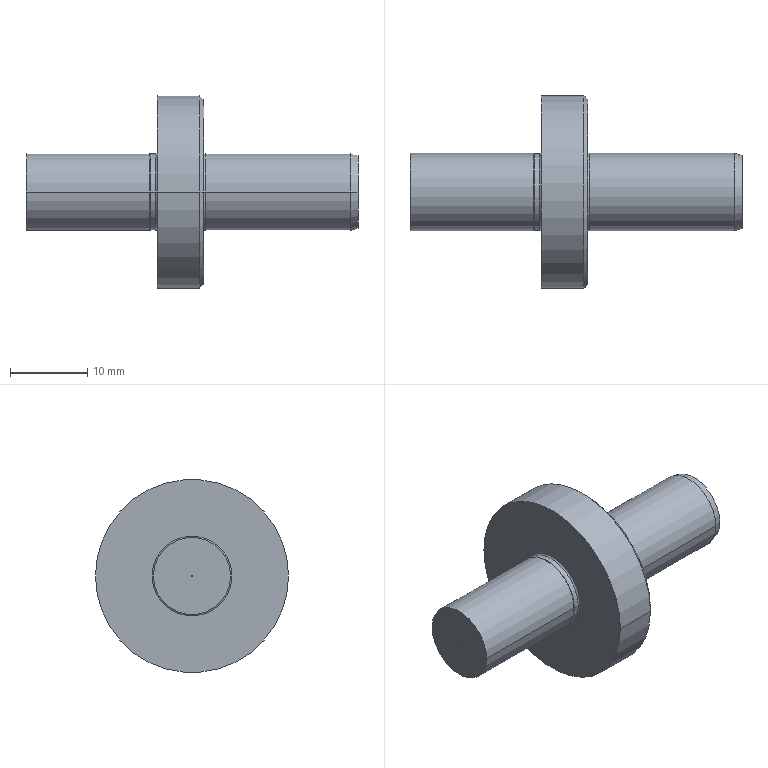Part | SolidWorks | features ICE 5, RevCut 5, Revolution 4, Fillet 2, Chamfer 1, DelFace 1, RefAxis 1 | 1 solid | 26 faces | box 43 x 25 x 25 mm | volume 5837 mm3 | cone 8 | cylinder 8 | torus 6 | plane 4 | commonest cylinder face diameters 10 x4 9.95 x2 25 x2
STEP:
#1=CARTESIAN_POINT('',(25.9,0.,0.));
#2=VERTEX_POINT('',#1);
#3=CARTESIAN_POINT('',(26.,0.,-0.1));
#4=VERTEX_POINT('',#3);
#5=CARTESIAN_POINT('',(26.,0.,-0.1));
#6=DIRECTION('',(0.7071,0.,-0.7071));
#7=VECTOR('',#6,1000.);
#8=LINE('',#5,#7);
#9=EDGE_CURVE('',#2,#4,#8,.T.);
#10=ORIENTED_EDGE('',*,*,#9,.F.);
#11=CARTESIAN_POINT('',(26.,0.,0.1));
#12=VERTEX_POINT('',#11);
#13=CARTESIAN_POINT('',(26.,0.,0.1));
#14=DIRECTION('',(0.7071,0.,0.7071));
#15=VECTOR('',#14,1000.);
#16=LINE('',#13,#15);
#17=EDGE_CURVE('',#2,#12,#16,.T.);
#18=ORIENTED_EDGE('',*,*,#17,.T.);
#19=CARTESIAN_POINT('',(26.,0.,0.));
#20=DIRECTION('',(-1.,0.,0.));
#21=DIRECTION('',(0.,0.,1.));
#22=AXIS2_PLACEMENT_3D('',#19,#20,#21);
#23=CIRCLE('',#22,0.1);
#24=EDGE_CURVE('',#4,#12,#23,.T.);
#25=ORIENTED_EDGE('',*,*,#24,.F.);
#26=EDGE_LOOP('',(#10,#18,#25));
#27=FACE_OUTER_BOUND('',#26,.T.);
#28=CARTESIAN_POINT('',(26.,0.,0.));
#29=DIRECTION('',(1.,0.,0.));
#30=DIRECTION('',(0.,0.,-1.));
#31=AXIS2_PLACEMENT_3D('',#28,#29,#30);
#32=CONICAL_SURFACE('',#31,0.1,0.7854);
#33=ADVANCED_FACE('',(#27),#32,.F.);
#34=CARTESIAN_POINT('',(26.,-4.732,0.));
#35=VERTEX_POINT('',#34);
#36=CARTESIAN_POINT('',(26.,4.732,0.));
#37=VERTEX_POINT('',#36);
#38=CARTESIAN_POINT('',(26.,0.,0.));
#39=DIRECTION('',(-1.,0.,0.));
#40=DIRECTION('',(0.,-1.,0.));
#41=AXIS2_PLACEMENT_3D('',#38,#39,#40);
#42=CIRCLE('',#41,4.732);
#43=EDGE_CURVE('',#35,#37,#42,.T.);
#44=ORIENTED_EDGE('',*,*,#43,.T.);
#45=CARTESIAN_POINT('',(25.,5.,0.));
#46=VERTEX_POINT('',#45);
#47=CARTESIAN_POINT('',(26.,4.732,0.));
#48=DIRECTION('',(-0.9659,0.2588,0.));
#49=VECTOR('',#48,1000.);
#50=LINE('',#47,#49);
#51=EDGE_CURVE('',#37,#46,#50,.T.);
#52=ORIENTED_EDGE('',*,*,#51,.T.);
#53=CARTESIAN_POINT('',(25.,-5.,0.));
#54=VERTEX_POINT('',#53);
#55=CARTESIAN_POINT('',(25.,0.,0.));
#56=DIRECTION('',(-1.,0.,0.));
#57=DIRECTION('',(0.,-1.,0.));
#58=AXIS2_PLACEMENT_3D('',#55,#56,#57);
#59=CIRCLE('',#58,5.);
#60=EDGE_CURVE('',#54,#46,#59,.T.);
#61=ORIENTED_EDGE('',*,*,#60,.F.);
#62=CARTESIAN_POINT('',(26.,-4.732,0.));
#63=DIRECTION('',(-0.9659,-0.2588,0.));
#64=VECTOR('',#63,1000.);
#65=LINE('',#62,#64);
#66=EDGE_CURVE('',#35,#54,#65,.T.);
#67=ORIENTED_EDGE('',*,*,#66,.F.);
#68=EDGE_LOOP('',(#44,#52,#61,#67));
#69=FACE_OUTER_BOUND('',#68,.T.);
#70=CARTESIAN_POINT('',(26.,0.,0.));
#71=DIRECTION('',(-1.,0.,0.));
#72=DIRECTION('',(0.,-1.,0.));
#73=AXIS2_PLACEMENT_3D('',#70,#71,#72);
#74=CONICAL_SURFACE('',#73,4.732,0.2618);
#75=ADVANCED_FACE('',(#69),#74,.T.);
#76=CARTESIAN_POINT('',(-1.,5.,0.));
#77=VERTEX_POINT('',#76);
#78=CARTESIAN_POINT('',(-1.,-5.,0.));
#79=VERTEX_POINT('',#78);
#80=CARTESIAN_POINT('',(-1.,0.,0.));
#81=DIRECTION('',(-1.,0.,0.));
#82=DIRECTION('',(0.,-1.,0.));
#83=AXIS2_PLACEMENT_3D('',#80,#81,#82);
#84=CIRCLE('',#83,5.);
#85=EDGE_CURVE('',#77,#79,#84,.T.);
#86=ORIENTED_EDGE('',*,*,#85,.F.);
#87=CARTESIAN_POINT('',(-0.9032,4.975,0.));
#88=VERTEX_POINT('',#87);
#89=CARTESIAN_POINT('',(-0.9032,5.175,0.));
#90=DIRECTION('',(0.,0.,1.));
#91=DIRECTION('',(0.,-1.,0.));
#92=AXIS2_PLACEMENT_3D('',#89,#90,#91);
#93=CIRCLE('',#92,0.2);
#94=EDGE_CURVE('',#77,#88,#93,.T.);
#95=ORIENTED_EDGE('',*,*,#94,.T.);
#96=CARTESIAN_POINT('',(-0.9032,-4.975,0.));
#97=VERTEX_POINT('',#96);
#98=CARTESIAN_POINT('',(-0.9032,0.,0.));
#99=DIRECTION('',(1.,0.,0.));
#100=DIRECTION('',(0.,-1.,0.));
#101=AXIS2_PLACEMENT_3D('',#98,#99,#100);
#102=CIRCLE('',#101,4.975);
#103=EDGE_CURVE('',#97,#88,#102,.T.);
#104=ORIENTED_EDGE('',*,*,#103,.F.);
#105=CARTESIAN_POINT('',(-0.9032,-5.175,0.));
#106=DIRECTION('',(0.,0.,-1.));
#107=DIRECTION('',(-1.,0.,0.));
#108=AXIS2_PLACEMENT_3D('',#105,#106,#107);
#109=CIRCLE('',#108,0.2);
#110=EDGE_CURVE('',#79,#97,#109,.T.);
#111=ORIENTED_EDGE('',*,*,#110,.F.);
#112=EDGE_LOOP('',(#86,#95,#104,#111));
#113=FACE_OUTER_BOUND('',#112,.T.);
#114=CARTESIAN_POINT('',(-0.9032,0.,0.));
#115=DIRECTION('',(-1.,0.,0.));
#116=DIRECTION('',(0.,-1.,0.));
#117=AXIS2_PLACEMENT_3D('',#114,#115,#116);
#118=TOROIDAL_SURFACE('',#117,5.175,0.2);
#119=ADVANCED_FACE('',(#113),#118,.F.);
#120=CARTESIAN_POINT('',(0.,-5.175,0.));
#121=VERTEX_POINT('',#120);
#122=CARTESIAN_POINT('',(0.,5.175,0.));
#123=VERTEX_POINT('',#122);
#124=CARTESIAN_POINT('',(0.,0.,0.));
#125=DIRECTION('',(1.,0.,0.));
#126=DIRECTION('',(0.,1.,0.));
#127=AXIS2_PLACEMENT_3D('',#124,#125,#126);
#128=CIRCLE('',#127,5.175);
#129=EDGE_CURVE('',#121,#123,#128,.T.);
#130=ORIENTED_EDGE('',*,*,#129,.F.);
#131=CARTESIAN_POINT('',(-0.2,-4.975,0.));
#132=VERTEX_POINT('',#131);
#133=CARTESIAN_POINT('',(-0.2,-5.175,0.));
#134=DIRECTION('',(0.,0.,1.));
#135=DIRECTION('',(0.,-1.,0.));
#136=AXIS2_PLACEMENT_3D('',#133,#134,#135);
#137=CIRCLE('',#136,0.2);
#138=EDGE_CURVE('',#121,#132,#137,.T.);
#139=ORIENTED_EDGE('',*,*,#138,.T.);
#140=CARTESIAN_POINT('',(-0.2,4.975,0.));
#141=VERTEX_POINT('',#140);
#142=CARTESIAN_POINT('',(-0.2,0.,0.));
#143=DIRECTION('',(-1.,0.,0.));
#144=DIRECTION('',(0.,1.,0.));
#145=AXIS2_PLACEMENT_3D('',#142,#143,#144);
#146=CIRCLE('',#145,4.975);
#147=EDGE_CURVE('',#141,#132,#146,.T.);
#148=ORIENTED_EDGE('',*,*,#147,.F.);
#149=CARTESIAN_POINT('',(-0.2,5.175,0.));
#150=DIRECTION('',(0.,0.,-1.));
#151=DIRECTION('',(-1.,0.,0.));
#152=AXIS2_PLACEMENT_3D('',#149,#150,#151);
#153=CIRCLE('',#152,0.2);
#154=EDGE_CURVE('',#123,#141,#153,.T.);
#155=ORIENTED_EDGE('',*,*,#154,.F.);
#156=EDGE_LOOP('',(#130,#139,#148,#155));
#157=FACE_OUTER_BOUND('',#156,.T.);
#158=CARTESIAN_POINT('',(-0.2,0.,0.));
#159=DIRECTION('',(1.,0.,0.));
#160=DIRECTION('',(0.,1.,0.));
#161=AXIS2_PLACEMENT_3D('',#158,#159,#160);
#162=TOROIDAL_SURFACE('',#161,5.175,0.2);
#163=ADVANCED_FACE('',(#157),#162,.F.);
#164=CARTESIAN_POINT('',(6.,5.2,0.));
#165=VERTEX_POINT('',#164);
#166=CARTESIAN_POINT('',(6.,-5.2,0.));
#167=VERTEX_POINT('',#166);
#168=CARTESIAN_POINT('',(6.,0.,0.));
#169=DIRECTION('',(-1.,0.,0.));
#170=DIRECTION('',(0.,-1.,0.));
#171=AXIS2_PLACEMENT_3D('',#168,#169,#170);
#172=CIRCLE('',#171,5.2);
#173=EDGE_CURVE('',#165,#167,#172,.T.);
#174=ORIENTED_EDGE('',*,*,#173,.F.);
#175=CARTESIAN_POINT('',(6.2,5.,0.));
#176=VERTEX_POINT('',#175);
#177=CARTESIAN_POINT('',(6.2,5.2,0.));
#178=DIRECTION('',(0.,0.,1.));
#179=DIRECTION('',(0.,-1.,0.));
#180=AXIS2_PLACEMENT_3D('',#177,#178,#179);
#181=CIRCLE('',#180,0.2);
#182=EDGE_CURVE('',#165,#176,#181,.T.);
#183=ORIENTED_EDGE('',*,*,#182,.T.);
#184=CARTESIAN_POINT('',(6.2,-5.,0.));
#185=VERTEX_POINT('',#184);
#186=CARTESIAN_POINT('',(6.2,0.,0.));
#187=DIRECTION('',(1.,0.,0.));
#188=DIRECTION('',(0.,-1.,0.));
#189=AXIS2_PLACEMENT_3D('',#186,#187,#188);
#190=CIRCLE('',#189,5.);
#191=EDGE_CURVE('',#185,#176,#190,.T.);
#192=ORIENTED_EDGE('',*,*,#191,.F.);
#193=CARTESIAN_POINT('',(6.2,-5.2,0.));
#194=DIRECTION('',(0.,0.,-1.));
#195=DIRECTION('',(-1.,0.,0.));
#196=AXIS2_PLACEMENT_3D('',#193,#194,#195);
#197=CIRCLE('',#196,0.2);
#198=EDGE_CURVE('',#167,#185,#197,.T.);
#199=ORIENTED_EDGE('',*,*,#198,.F.);
#200=EDGE_LOOP('',(#174,#183,#192,#199));
#201=FACE_OUTER_BOUND('',#200,.T.);
#202=CARTESIAN_POINT('',(6.2,0.,0.));
#203=DIRECTION('',(-1.,0.,0.));
#204=DIRECTION('',(0.,-1.,0.));
#205=AXIS2_PLACEMENT_3D('',#202,#203,#204);
#206=TOROIDAL_SURFACE('',#205,5.2,0.2);
#207=ADVANCED_FACE('',(#201),#206,.F.);
#208=CARTESIAN_POINT('',(6.,12.,0.));
#209=VERTEX_POINT('',#208);
#210=CARTESIAN_POINT('',(6.,-12.,0.));
#211=VERTEX_POINT('',#210);
#212=CARTESIAN_POINT('',(6.,0.,0.));
#213=DIRECTION('',(1.,0.,0.));
#214=DIRECTION('',(0.,-1.,0.));
#215=AXIS2_PLACEMENT_3D('',#212,#213,#214);
#216=CIRCLE('',#215,12.);
#217=EDGE_CURVE('',#209,#211,#216,.T.);
#218=ORIENTED_EDGE('',*,*,#217,.F.);
#219=CARTESIAN_POINT('',(5.5,12.5,0.));
#220=VERTEX_POINT('',#219);
#221=CARTESIAN_POINT('',(5.5,12.5,0.));
#222=DIRECTION('',(-0.7071,0.7071,0.));
#223=VECTOR('',#222,1000.);
#224=LINE('',#221,#223);
#225=EDGE_CURVE('',#209,#220,#224,.T.);
#226=ORIENTED_EDGE('',*,*,#225,.T.);
#227=CARTESIAN_POINT('',(5.5,-12.5,0.));
#228=VERTEX_POINT('',#227);
#229=CARTESIAN_POINT('',(5.5,0.,0.));
#230=DIRECTION('',(-1.,0.,0.));
#231=DIRECTION('',(0.,-1.,0.));
#232=AXIS2_PLACEMENT_3D('',#229,#230,#231);
#233=CIRCLE('',#232,12.5);
#234=EDGE_CURVE('',#228,#220,#233,.T.);
#235=ORIENTED_EDGE('',*,*,#234,.F.);
#236=CARTESIAN_POINT('',(5.5,-12.5,0.));
#237=DIRECTION('',(-0.7071,-0.7071,0.));
#238=VECTOR('',#237,1000.);
#239=LINE('',#236,#238);
#240=EDGE_CURVE('',#211,#228,#239,.T.);
#241=ORIENTED_EDGE('',*,*,#240,.F.);
#242=EDGE_LOOP('',(#218,#226,#235,#241));
#243=FACE_OUTER_BOUND('',#242,.T.);
#244=CARTESIAN_POINT('',(5.5,0.,0.));
#245=DIRECTION('',(-1.,0.,0.));
#246=DIRECTION('',(0.,-1.,0.));
#247=AXIS2_PLACEMENT_3D('',#244,#245,#246);
#248=CONICAL_SURFACE('',#247,12.5,0.7854);
#249=ADVANCED_FACE('',(#243),#248,.T.);
#250=CARTESIAN_POINT('',(-16.9,0.,0.));
#251=VERTEX_POINT('',#250);
#252=CARTESIAN_POINT('',(-17.,0.,0.1));
#253=VERTEX_POINT('',#252);
#254=CARTESIAN_POINT('',(-16.9,0.,0.));
#255=DIRECTION('',(-0.7071,0.,0.7071));
#256=VECTOR('',#255,1000.);
#257=LINE('',#254,#256);
#258=EDGE_CURVE('',#251,#253,#257,.T.);
#259=ORIENTED_EDGE('',*,*,#258,.F.);
#260=CARTESIAN_POINT('',(-17.,0.,-0.1));
#261=VERTEX_POINT('',#260);
#262=CARTESIAN_POINT('',(-16.9,0.,0.));
#263=DIRECTION('',(-0.7071,0.,-0.7071));
#264=VECTOR('',#263,1000.);
#265=LINE('',#262,#264);
#266=EDGE_CURVE('',#251,#261,#265,.T.);
#267=ORIENTED_EDGE('',*,*,#266,.T.);
#268=CARTESIAN_POINT('',(-17.,0.,0.));
#269=DIRECTION('',(-1.,0.,0.));
#270=DIRECTION('',(0.,0.,1.));
#271=AXIS2_PLACEMENT_3D('',#268,#269,#270);
#272=CIRCLE('',#271,0.1);
#273=EDGE_CURVE('',#261,#253,#272,.T.);
#274=ORIENTED_EDGE('',*,*,#273,.T.);
#275=EDGE_LOOP('',(#259,#267,#274));
#276=FACE_OUTER_BOUND('',#275,.T.);
#277=CARTESIAN_POINT('',(-1016.9,0.,0.));
#278=DIRECTION('',(-1.,0.,0.));
#279=DIRECTION('',(0.,0.,1.));
#280=AXIS2_PLACEMENT_3D('',#277,#278,#279);
#281=CONICAL_SURFACE('',#280,1000.,0.7854);
#282=ADVANCED_FACE('',(#276),#281,.F.);
#283=ORIENTED_EDGE('',*,*,#60,.T.);
#284=CARTESIAN_POINT('',(-17.,5.,0.));
#285=DIRECTION('',(-1.,0.,0.));
#286=VECTOR('',#285,1000.);
#287=LINE('',#284,#286);
#288=EDGE_CURVE('',#46,#176,#287,.T.);
#289=ORIENTED_EDGE('',*,*,#288,.T.);
#290=CARTESIAN_POINT('',(6.2,0.,0.));
#291=DIRECTION('',(1.,0.,0.));
#292=DIRECTION('',(0.,-1.,0.));
#293=AXIS2_PLACEMENT_3D('',#290,#291,#292);
#294=CIRCLE('',#293,5.);
#295=EDGE_CURVE('',#176,#185,#294,.T.);
#296=ORIENTED_EDGE('',*,*,#295,.T.);
#297=CARTESIAN_POINT('',(-17.,-5.,0.));
#298=DIRECTION('',(-1.,0.,0.));
#299=VECTOR('',#298,1000.);
#300=LINE('',#297,#299);
#301=EDGE_CURVE('',#54,#185,#300,.T.);
#302=ORIENTED_EDGE('',*,*,#301,.F.);
#303=EDGE_LOOP('',(#283,#289,#296,#302));
#304=FACE_OUTER_BOUND('',#303,.T.);
#305=CARTESIAN_POINT('',(-17.,0.,0.));
#306=DIRECTION('',(-1.,0.,0.));
#307=DIRECTION('',(0.,-1.,0.));
#308=AXIS2_PLACEMENT_3D('',#305,#306,#307);
#309=CYLINDRICAL_SURFACE('',#308,5.);
#310=ADVANCED_FACE('',(#304),#309,.T.);
#311=ORIENTED_EDGE('',*,*,#234,.T.);
#312=CARTESIAN_POINT('',(0.,12.5,0.));
#313=VERTEX_POINT('',#312);
#314=CARTESIAN_POINT('',(-17.,12.5,0.));
#315=DIRECTION('',(-1.,0.,0.));
#316=VECTOR('',#315,1000.);
#317=LINE('',#314,#316);
#318=EDGE_CURVE('',#220,#313,#317,.T.);
#319=ORIENTED_EDGE('',*,*,#318,.T.);
#320=CARTESIAN_POINT('',(0.,-12.5,0.));
#321=VERTEX_POINT('',#320);
#322=CARTESIAN_POINT('',(0.,0.,0.));
#323=DIRECTION('',(-1.,0.,0.));
#324=DIRECTION('',(0.,-1.,0.));
#325=AXIS2_PLACEMENT_3D('',#322,#323,#324);
#326=CIRCLE('',#325,12.5);
#327=EDGE_CURVE('',#321,#313,#326,.T.);
#328=ORIENTED_EDGE('',*,*,#327,.F.);
#329=CARTESIAN_POINT('',(-17.,-12.5,0.));
#330=DIRECTION('',(-1.,0.,0.));
#331=VECTOR('',#330,1000.);
#332=LINE('',#329,#331);
#333=EDGE_CURVE('',#228,#321,#332,.T.);
#334=ORIENTED_EDGE('',*,*,#333,.F.);
#335=EDGE_LOOP('',(#311,#319,#328,#334));
#336=FACE_OUTER_BOUND('',#335,.T.);
#337=CARTESIAN_POINT('',(-17.,0.,0.));
#338=DIRECTION('',(-1.,0.,0.));
#339=DIRECTION('',(0.,-1.,0.));
#340=AXIS2_PLACEMENT_3D('',#337,#338,#339);
#341=CYLINDRICAL_SURFACE('',#340,12.5);
#342=ADVANCED_FACE('',(#336),#341,.T.);
#343=CARTESIAN_POINT('',(-0.2,0.,0.));
#344=DIRECTION('',(-1.,0.,0.));
#345=DIRECTION('',(0.,1.,0.));
#346=AXIS2_PLACEMENT_3D('',#343,#344,#345);
#347=CIRCLE('',#346,4.975);
#348=EDGE_CURVE('',#132,#141,#347,.T.);
#349=ORIENTED_EDGE('',*,*,#348,.T.);
#350=CARTESIAN_POINT('',(-17.,4.975,0.));
#351=DIRECTION('',(-1.,0.,0.));
#352=VECTOR('',#351,1000.);
#353=LINE('',#350,#352);
#354=EDGE_CURVE('',#141,#88,#353,.T.);
#355=ORIENTED_EDGE('',*,*,#354,.T.);
#356=CARTESIAN_POINT('',(-0.9032,0.,0.));
#357=DIRECTION('',(1.,0.,0.));
#358=DIRECTION('',(0.,-1.,0.));
#359=AXIS2_PLACEMENT_3D('',#356,#357,#358);
#360=CIRCLE('',#359,4.975);
#361=EDGE_CURVE('',#88,#97,#360,.T.);
#362=ORIENTED_EDGE('',*,*,#361,.T.);
#363=CARTESIAN_POINT('',(-17.,-4.975,0.));
#364=DIRECTION('',(-1.,0.,0.));
#365=VECTOR('',#364,1000.);
#366=LINE('',#363,#365);
#367=EDGE_CURVE('',#132,#97,#366,.T.);
#368=ORIENTED_EDGE('',*,*,#367,.F.);
#369=EDGE_LOOP('',(#349,#355,#362,#368));
#370=FACE_OUTER_BOUND('',#369,.T.);
#371=CARTESIAN_POINT('',(-17.,0.,0.));
#372=DIRECTION('',(-1.,0.,0.));
#373=DIRECTION('',(0.,-1.,0.));
#374=AXIS2_PLACEMENT_3D('',#371,#372,#373);
#375=CYLINDRICAL_SURFACE('',#374,4.975);
#376=ADVANCED_FACE('',(#370),#375,.T.);
#377=CARTESIAN_POINT('',(-1.,0.,0.));
#378=DIRECTION('',(-1.,0.,0.));
#379=DIRECTION('',(0.,-1.,0.));
#380=AXIS2_PLACEMENT_3D('',#377,#378,#379);
#381=CIRCLE('',#380,5.);
#382=EDGE_CURVE('',#79,#77,#381,.T.);
#383=ORIENTED_EDGE('',*,*,#382,.T.);
#384=CARTESIAN_POINT('',(-17.,5.,0.));
#385=VERTEX_POINT('',#384);
#386=CARTESIAN_POINT('',(-17.,5.,0.));
#387=DIRECTION('',(-1.,0.,0.));
#388=VECTOR('',#387,1000.);
#389=LINE('',#386,#388);
#390=EDGE_CURVE('',#77,#385,#389,.T.);
#391=ORIENTED_EDGE('',*,*,#390,.T.);
#392=CARTESIAN_POINT('',(-17.,-5.,0.));
#393=VERTEX_POINT('',#392);
#394=CARTESIAN_POINT('',(-17.,0.,0.));
#395=DIRECTION('',(-1.,0.,0.));
#396=DIRECTION('',(0.,-1.,0.));
#397=AXIS2_PLACEMENT_3D('',#394,#395,#396);
#398=CIRCLE('',#397,5.);
#399=EDGE_CURVE('',#393,#385,#398,.T.);
#400=ORIENTED_EDGE('',*,*,#399,.F.);
#401=CARTESIAN_POINT('',(-17.,-5.,0.));
#402=DIRECTION('',(-1.,0.,0.));
#403=VECTOR('',#402,1000.);
#404=LINE('',#401,#403);
#405=EDGE_CURVE('',#79,#393,#404,.T.);
#406=ORIENTED_EDGE('',*,*,#405,.F.);
#407=EDGE_LOOP('',(#383,#391,#400,#406));
#408=FACE_OUTER_BOUND('',#407,.T.);
#409=CARTESIAN_POINT('',(-17.,0.,0.));
#410=DIRECTION('',(-1.,0.,0.));
#411=DIRECTION('',(0.,-1.,0.));
#412=AXIS2_PLACEMENT_3D('',#409,#410,#411);
#413=CYLINDRICAL_SURFACE('',#412,5.);
#414=ADVANCED_FACE('',(#408),#413,.T.);
#415=ORIENTED_EDGE('',*,*,#43,.F.);
#416=CARTESIAN_POINT('',(26.,0.,0.));
#417=DIRECTION('',(-1.,0.,0.));
#418=DIRECTION('',(0.,-1.,0.));
#419=AXIS2_PLACEMENT_3D('',#416,#417,#418);
#420=CIRCLE('',#419,4.732);
#421=EDGE_CURVE('',#37,#35,#420,.T.);
#422=ORIENTED_EDGE('',*,*,#421,.F.);
#423=EDGE_LOOP('',(#415,#422));
#424=FACE_OUTER_BOUND('',#423,.T.);
#425=ORIENTED_EDGE('',*,*,#24,.T.);
#426=CARTESIAN_POINT('',(26.,0.,0.));
#427=DIRECTION('',(-1.,0.,0.));
#428=DIRECTION('',(0.,0.,1.));
#429=AXIS2_PLACEMENT_3D('',#426,#427,#428);
#430=CIRCLE('',#429,0.1);
#431=EDGE_CURVE('',#12,#4,#430,.T.);
#432=ORIENTED_EDGE('',*,*,#431,.T.);
#433=EDGE_LOOP('',(#425,#432));
#434=FACE_BOUND('',#433,.T.);
#435=CARTESIAN_POINT('',(26.,4.732,0.));
#436=DIRECTION('',(-1.,0.,0.));
#437=DIRECTION('',(0.,-1.,0.));
#438=AXIS2_PLACEMENT_3D('',#435,#436,#437);
#439=PLANE('',#438);
#440=ADVANCED_FACE('',(#424,#434),#439,.F.);
#441=ORIENTED_EDGE('',*,*,#399,.T.);
#442=CARTESIAN_POINT('',(-17.,0.,0.));
#443=DIRECTION('',(-1.,0.,0.));
#444=DIRECTION('',(0.,-1.,0.));
#445=AXIS2_PLACEMENT_3D('',#442,#443,#444);
#446=CIRCLE('',#445,5.);
#447=EDGE_CURVE('',#385,#393,#446,.T.);
#448=ORIENTED_EDGE('',*,*,#447,.T.);
#449=EDGE_LOOP('',(#441,#448));
#450=FACE_OUTER_BOUND('',#449,.T.);
#451=CARTESIAN_POINT('',(-17.,0.,0.));
#452=DIRECTION('',(-1.,0.,0.));
#453=DIRECTION('',(0.,0.,1.));
#454=AXIS2_PLACEMENT_3D('',#451,#452,#453);
#455=CIRCLE('',#454,0.1);
#456=EDGE_CURVE('',#253,#261,#455,.T.);
#457=ORIENTED_EDGE('',*,*,#456,.F.);
#458=ORIENTED_EDGE('',*,*,#273,.F.);
#459=EDGE_LOOP('',(#457,#458));
#460=FACE_BOUND('',#459,.T.);
#461=CARTESIAN_POINT('',(-17.,0.,0.));
#462=DIRECTION('',(1.,0.,0.));
#463=DIRECTION('',(0.,1.,0.));
#464=AXIS2_PLACEMENT_3D('',#461,#462,#463);
#465=PLANE('',#464);
#466=ADVANCED_FACE('',(#450,#460),#465,.F.);
#467=ORIENTED_EDGE('',*,*,#390,.F.);
#468=ORIENTED_EDGE('',*,*,#85,.T.);
#469=ORIENTED_EDGE('',*,*,#405,.T.);
#470=ORIENTED_EDGE('',*,*,#447,.F.);
#471=EDGE_LOOP('',(#467,#468,#469,#470));
#472=FACE_OUTER_BOUND('',#471,.T.);
#473=CARTESIAN_POINT('',(-17.,0.,0.));
#474=DIRECTION('',(-1.,0.,0.));
#475=DIRECTION('',(0.,-1.,0.));
#476=AXIS2_PLACEMENT_3D('',#473,#474,#475);
#477=CYLINDRICAL_SURFACE('',#476,5.);
#478=ADVANCED_FACE('',(#472),#477,.T.);
#479=ORIENTED_EDGE('',*,*,#354,.F.);
#480=ORIENTED_EDGE('',*,*,#147,.T.);
#481=ORIENTED_EDGE('',*,*,#367,.T.);
#482=ORIENTED_EDGE('',*,*,#103,.T.);
#483=EDGE_LOOP('',(#479,#480,#481,#482));
#484=FACE_OUTER_BOUND('',#483,.T.);
#485=CARTESIAN_POINT('',(-17.,0.,0.));
#486=DIRECTION('',(-1.,0.,0.));
#487=DIRECTION('',(0.,-1.,0.));
#488=AXIS2_PLACEMENT_3D('',#485,#486,#487);
#489=CYLINDRICAL_SURFACE('',#488,4.975);
#490=ADVANCED_FACE('',(#484),#489,.T.);
#491=CARTESIAN_POINT('',(0.,0.,0.));
#492=DIRECTION('',(1.,0.,0.));
#493=DIRECTION('',(0.,1.,0.));
#494=AXIS2_PLACEMENT_3D('',#491,#492,#493);
#495=CIRCLE('',#494,5.175);
#496=EDGE_CURVE('',#123,#121,#495,.T.);
#497=ORIENTED_EDGE('',*,*,#496,.T.);
#498=ORIENTED_EDGE('',*,*,#129,.T.);
#499=EDGE_LOOP('',(#497,#498));
#500=FACE_BOUND('',#499,.T.);
#501=ORIENTED_EDGE('',*,*,#327,.T.);
#502=CARTESIAN_POINT('',(0.,0.,0.));
#503=DIRECTION('',(-1.,0.,0.));
#504=DIRECTION('',(0.,-1.,0.));
#505=AXIS2_PLACEMENT_3D('',#502,#503,#504);
#506=CIRCLE('',#505,12.5);
#507=EDGE_CURVE('',#313,#321,#506,.T.);
#508=ORIENTED_EDGE('',*,*,#507,.T.);
#509=EDGE_LOOP('',(#501,#508));
#510=FACE_OUTER_BOUND('',#509,.T.);
#511=CARTESIAN_POINT('',(0.,4.975,0.));
#512=DIRECTION('',(1.,0.,0.));
#513=DIRECTION('',(0.,1.,0.));
#514=AXIS2_PLACEMENT_3D('',#511,#512,#513);
#515=PLANE('',#514);
#516=ADVANCED_FACE('',(#500,#510),#515,.F.);
#517=ORIENTED_EDGE('',*,*,#318,.F.);
#518=CARTESIAN_POINT('',(5.5,0.,0.));
#519=DIRECTION('',(-1.,0.,0.));
#520=DIRECTION('',(0.,-1.,0.));
#521=AXIS2_PLACEMENT_3D('',#518,#519,#520);
#522=CIRCLE('',#521,12.5);
#523=EDGE_CURVE('',#220,#228,#522,.T.);
#524=ORIENTED_EDGE('',*,*,#523,.T.);
#525=ORIENTED_EDGE('',*,*,#333,.T.);
#526=ORIENTED_EDGE('',*,*,#507,.F.);
#527=EDGE_LOOP('',(#517,#524,#525,#526));
#528=FACE_OUTER_BOUND('',#527,.T.);
#529=CARTESIAN_POINT('',(-17.,0.,0.));
#530=DIRECTION('',(-1.,0.,0.));
#531=DIRECTION('',(0.,-1.,0.));
#532=AXIS2_PLACEMENT_3D('',#529,#530,#531);
#533=CYLINDRICAL_SURFACE('',#532,12.5);
#534=ADVANCED_FACE('',(#528),#533,.T.);
#535=CARTESIAN_POINT('',(6.,0.,0.));
#536=DIRECTION('',(-1.,0.,0.));
#537=DIRECTION('',(0.,-1.,0.));
#538=AXIS2_PLACEMENT_3D('',#535,#536,#537);
#539=CIRCLE('',#538,5.2);
#540=EDGE_CURVE('',#167,#165,#539,.T.);
#541=ORIENTED_EDGE('',*,*,#540,.T.);
#542=ORIENTED_EDGE('',*,*,#173,.T.);
#543=EDGE_LOOP('',(#541,#542));
#544=FACE_BOUND('',#543,.T.);
#545=CARTESIAN_POINT('',(6.,0.,0.));
#546=DIRECTION('',(1.,0.,0.));
#547=DIRECTION('',(0.,-1.,0.));
#548=AXIS2_PLACEMENT_3D('',#545,#546,#547);
#549=CIRCLE('',#548,12.);
#550=EDGE_CURVE('',#211,#209,#549,.T.);
#551=ORIENTED_EDGE('',*,*,#550,.T.);
#552=ORIENTED_EDGE('',*,*,#217,.T.);
#553=EDGE_LOOP('',(#551,#552));
#554=FACE_OUTER_BOUND('',#553,.T.);
#555=CARTESIAN_POINT('',(6.,12.5,0.));
#556=DIRECTION('',(-1.,0.,0.));
#557=DIRECTION('',(0.,-1.,0.));
#558=AXIS2_PLACEMENT_3D('',#555,#556,#557);
#559=PLANE('',#558);
#560=ADVANCED_FACE('',(#544,#554),#559,.F.);
#561=ORIENTED_EDGE('',*,*,#288,.F.);
#562=CARTESIAN_POINT('',(25.,0.,0.));
#563=DIRECTION('',(-1.,0.,0.));
#564=DIRECTION('',(0.,-1.,0.));
#565=AXIS2_PLACEMENT_3D('',#562,#563,#564);
#566=CIRCLE('',#565,5.);
#567=EDGE_CURVE('',#46,#54,#566,.T.);
#568=ORIENTED_EDGE('',*,*,#567,.T.);
#569=ORIENTED_EDGE('',*,*,#301,.T.);
#570=ORIENTED_EDGE('',*,*,#191,.T.);
#571=EDGE_LOOP('',(#561,#568,#569,#570));
#572=FACE_OUTER_BOUND('',#571,.T.);
#573=CARTESIAN_POINT('',(-17.,0.,0.));
#574=DIRECTION('',(-1.,0.,0.));
#575=DIRECTION('',(0.,-1.,0.));
#576=AXIS2_PLACEMENT_3D('',#573,#574,#575);
#577=CYLINDRICAL_SURFACE('',#576,5.);
#578=ADVANCED_FACE('',(#572),#577,.T.);
#579=ORIENTED_EDGE('',*,*,#266,.F.);
#580=ORIENTED_EDGE('',*,*,#258,.T.);
#581=ORIENTED_EDGE('',*,*,#456,.T.);
#582=EDGE_LOOP('',(#579,#580,#581));
#583=FACE_OUTER_BOUND('',#582,.T.);
#584=CARTESIAN_POINT('',(-1016.9,0.,0.));
#585=DIRECTION('',(-1.,0.,0.));
#586=DIRECTION('',(0.,0.,1.));
#587=AXIS2_PLACEMENT_3D('',#584,#585,#586);
#588=CONICAL_SURFACE('',#587,1000.,0.7854);
#589=ADVANCED_FACE('',(#583),#588,.F.);
#590=ORIENTED_EDGE('',*,*,#225,.F.);
#591=ORIENTED_EDGE('',*,*,#550,.F.);
#592=ORIENTED_EDGE('',*,*,#240,.T.);
#593=ORIENTED_EDGE('',*,*,#523,.F.);
#594=EDGE_LOOP('',(#590,#591,#592,#593));
#595=FACE_OUTER_BOUND('',#594,.T.);
#596=CARTESIAN_POINT('',(5.5,0.,0.));
#597=DIRECTION('',(-1.,0.,0.));
#598=DIRECTION('',(0.,-1.,0.));
#599=AXIS2_PLACEMENT_3D('',#596,#597,#598);
#600=CONICAL_SURFACE('',#599,12.5,0.7854);
#601=ADVANCED_FACE('',(#595),#600,.T.);
#602=ORIENTED_EDGE('',*,*,#182,.F.);
#603=ORIENTED_EDGE('',*,*,#540,.F.);
#604=ORIENTED_EDGE('',*,*,#198,.T.);
#605=ORIENTED_EDGE('',*,*,#295,.F.);
#606=EDGE_LOOP('',(#602,#603,#604,#605));
#607=FACE_OUTER_BOUND('',#606,.T.);
#608=CARTESIAN_POINT('',(6.2,0.,0.));
#609=DIRECTION('',(-1.,0.,0.));
#610=DIRECTION('',(0.,-1.,0.));
#611=AXIS2_PLACEMENT_3D('',#608,#609,#610);
#612=TOROIDAL_SURFACE('',#611,5.2,0.2);
#613=ADVANCED_FACE('',(#607),#612,.F.);
#614=ORIENTED_EDGE('',*,*,#138,.F.);
#615=ORIENTED_EDGE('',*,*,#496,.F.);
#616=ORIENTED_EDGE('',*,*,#154,.T.);
#617=ORIENTED_EDGE('',*,*,#348,.F.);
#618=EDGE_LOOP('',(#614,#615,#616,#617));
#619=FACE_OUTER_BOUND('',#618,.T.);
#620=CARTESIAN_POINT('',(-0.2,0.,0.));
#621=DIRECTION('',(1.,0.,0.));
#622=DIRECTION('',(0.,1.,0.));
#623=AXIS2_PLACEMENT_3D('',#620,#621,#622);
#624=TOROIDAL_SURFACE('',#623,5.175,0.2);
#625=ADVANCED_FACE('',(#619),#624,.F.);
#626=ORIENTED_EDGE('',*,*,#94,.F.);
#627=ORIENTED_EDGE('',*,*,#382,.F.);
#628=ORIENTED_EDGE('',*,*,#110,.T.);
#629=ORIENTED_EDGE('',*,*,#361,.F.);
#630=EDGE_LOOP('',(#626,#627,#628,#629));
#631=FACE_OUTER_BOUND('',#630,.T.);
#632=CARTESIAN_POINT('',(-0.9032,0.,0.));
#633=DIRECTION('',(-1.,0.,0.));
#634=DIRECTION('',(0.,-1.,0.));
#635=AXIS2_PLACEMENT_3D('',#632,#633,#634);
#636=TOROIDAL_SURFACE('',#635,5.175,0.2);
#637=ADVANCED_FACE('',(#631),#636,.F.);
#638=ORIENTED_EDGE('',*,*,#51,.F.);
#639=ORIENTED_EDGE('',*,*,#421,.T.);
#640=ORIENTED_EDGE('',*,*,#66,.T.);
#641=ORIENTED_EDGE('',*,*,#567,.F.);
#642=EDGE_LOOP('',(#638,#639,#640,#641));
#643=FACE_OUTER_BOUND('',#642,.T.);
#644=CARTESIAN_POINT('',(26.,0.,0.));
#645=DIRECTION('',(-1.,0.,0.));
#646=DIRECTION('',(0.,-1.,0.));
#647=AXIS2_PLACEMENT_3D('',#644,#645,#646);
#648=CONICAL_SURFACE('',#647,4.732,0.2618);
#649=ADVANCED_FACE('',(#643),#648,.T.);
#650=ORIENTED_EDGE('',*,*,#17,.F.);
#651=ORIENTED_EDGE('',*,*,#9,.T.);
#652=ORIENTED_EDGE('',*,*,#431,.F.);
#653=EDGE_LOOP('',(#650,#651,#652));
#654=FACE_OUTER_BOUND('',#653,.T.);
#655=CARTESIAN_POINT('',(26.,0.,0.));
#656=DIRECTION('',(1.,0.,0.));
#657=DIRECTION('',(0.,0.,-1.));
#658=AXIS2_PLACEMENT_3D('',#655,#656,#657);
#659=CONICAL_SURFACE('',#658,0.1,0.7854);
#660=ADVANCED_FACE('',(#654),#659,.F.);
#661=CLOSED_SHELL('',(#33,#75,#119,#163,#207,#249,#282,#310,#342,#376,#414,#440,#466,#478,#490,#516,#534,#560,#578,#589,#601,#613,#625,#637,#649,#660));
#662=MANIFOLD_SOLID_BREP('',#661);
#663=CARTESIAN_POINT('',(0.,0.,0.));
#664=DIRECTION('',(0.,0.,1.));
#665=DIRECTION('',(1.,0.,0.));
#666=AXIS2_PLACEMENT_3D('',#663,#664,#665);
#667=(LENGTH_UNIT()NAMED_UNIT(*)SI_UNIT(.MILLI.,.METRE.));
#668=UNCERTAINTY_MEASURE_WITH_UNIT(LENGTH_MEASURE(0.00001),#667,'','');
#669=(NAMED_UNIT(*)PLANE_ANGLE_UNIT()SI_UNIT($,.RADIAN.));
#670=(NAMED_UNIT(*)SI_UNIT($,.STERADIAN.)SOLID_ANGLE_UNIT());
#671=(GEOMETRIC_REPRESENTATION_CONTEXT(3)GLOBAL_UNCERTAINTY_ASSIGNED_CONTEXT((#668))GLOBAL_UNIT_ASSIGNED_CONTEXT((#667,#669,#670))REPRESENTATION_CONTEXT('',''));
#672=ADVANCED_BREP_SHAPE_REPRESENTATION('',(#662,#666),#671);